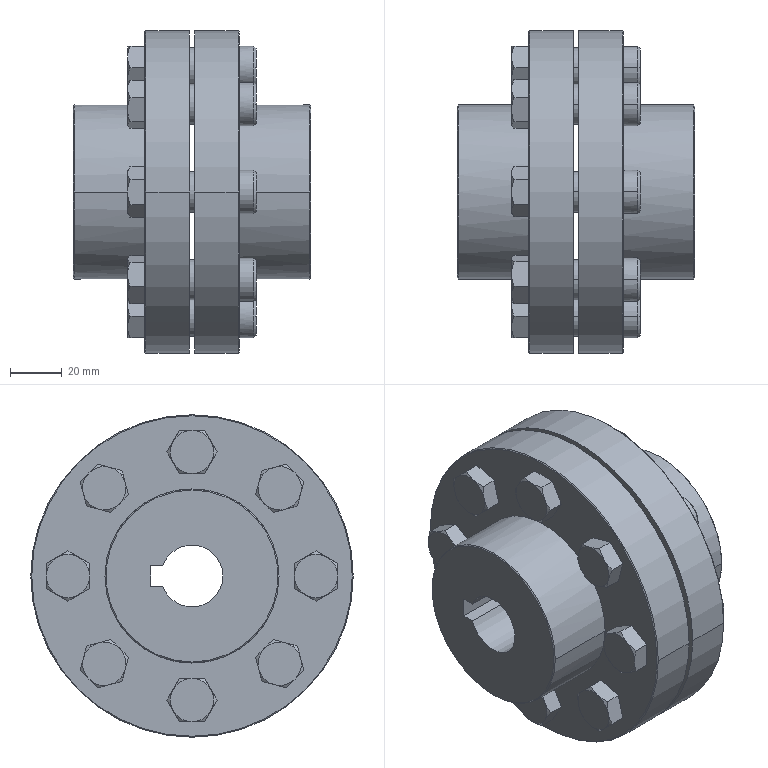Part | SolidWorks | features ICE 4, Chamfer 2, BaseBody 1, Scale 1 | 1 solid | 229 faces | box 92 x 125 x 125 mm | volume 604795 mm3 | plane 92 | cone 75 | cylinder 62 | commonest cylinder face diameters 12.48 x16 15.6 x16 16.8 x16 24 x4 67.5 x4 125 x4